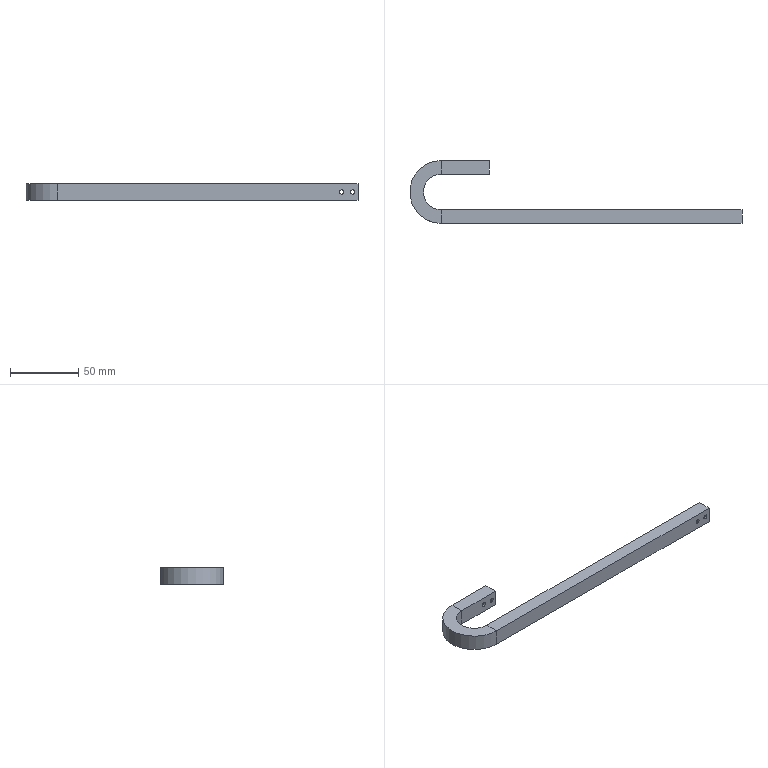Part | NX | features BREP 1 | 1 solid | 46 faces | box 243 x 46 x 12 mm | volume 22023 mm3 | plane 22 | cylinder 20 | cone 4 | commonest cylinder face diameters 3.2 x16 26 x1 29 x1 43 x1 46 x1
STEP:
#1=CARTESIAN_POINT('',(181.,-39.5,-1.6));
#2=VERTEX_POINT('',#1);
#3=CARTESIAN_POINT('',(181.,-40.999,-1.6));
#4=VERTEX_POINT('',#3);
#5=CARTESIAN_POINT('',(181.,-31.,-1.6));
#6=DIRECTION('',(0.,1.,0.));
#7=VECTOR('',#6,1000.);
#8=LINE('',#5,#7);
#9=EDGE_CURVE('',#2,#4,#8,.F.);
#10=ORIENTED_EDGE('',*,*,#9,.T.);
#11=CARTESIAN_POINT('',(181.,-40.999,1.6));
#12=VERTEX_POINT('',#11);
#13=CARTESIAN_POINT('',(181.,-40.999,0.));
#14=DIRECTION('',(0.,1.,0.));
#15=DIRECTION('',(0.,0.,1.));
#16=AXIS2_PLACEMENT_3D('',#13,#14,#15);
#17=CIRCLE('',#16,1.6);
#18=EDGE_CURVE('',#12,#4,#17,.T.);
#19=ORIENTED_EDGE('',*,*,#18,.F.);
#20=CARTESIAN_POINT('',(181.,-39.5,1.6));
#21=VERTEX_POINT('',#20);
#22=CARTESIAN_POINT('',(181.,-31.,1.6));
#23=DIRECTION('',(0.,1.,0.));
#24=VECTOR('',#23,1000.);
#25=LINE('',#22,#24);
#26=EDGE_CURVE('',#21,#12,#25,.F.);
#27=ORIENTED_EDGE('',*,*,#26,.F.);
#28=CARTESIAN_POINT('',(181.,-39.5,0.));
#29=DIRECTION('',(0.,-1.,0.));
#30=DIRECTION('',(1.,0.,0.));
#31=AXIS2_PLACEMENT_3D('',#28,#29,#30);
#32=CIRCLE('',#31,1.6);
#33=EDGE_CURVE('',#2,#21,#32,.T.);
#34=ORIENTED_EDGE('',*,*,#33,.F.);
#35=EDGE_LOOP('',(#10,#19,#27,#34));
#36=FACE_BOUND('',#35,.T.);
#37=CARTESIAN_POINT('',(181.,-31.,0.));
#38=DIRECTION('',(0.,1.,0.));
#39=DIRECTION('',(0.,0.,1.));
#40=AXIS2_PLACEMENT_3D('',#37,#38,#39);
#41=CYLINDRICAL_SURFACE('',#40,1.6);
#42=ADVANCED_FACE('',(#36),#41,.F.);
#43=CARTESIAN_POINT('',(181.,-41.,-1.598));
#44=VERTEX_POINT('',#43);
#45=CARTESIAN_POINT('',(181.,-40.999,-1.6));
#46=DIRECTION('',(0.,0.515,-0.8572));
#47=VECTOR('',#46,1000.);
#48=LINE('',#45,#47);
#49=EDGE_CURVE('',#4,#44,#48,.F.);
#50=ORIENTED_EDGE('',*,*,#49,.T.);
#51=CARTESIAN_POINT('',(181.,-41.,1.598));
#52=VERTEX_POINT('',#51);
#53=CARTESIAN_POINT('',(181.,-41.,0.));
#54=DIRECTION('',(0.,1.,0.));
#55=DIRECTION('',(-1.,0.,0.));
#56=AXIS2_PLACEMENT_3D('',#53,#54,#55);
#57=CIRCLE('',#56,1.598);
#58=EDGE_CURVE('',#52,#44,#57,.T.);
#59=ORIENTED_EDGE('',*,*,#58,.F.);
#60=CARTESIAN_POINT('',(181.,-40.999,1.6));
#61=DIRECTION('',(0.,0.515,0.8572));
#62=VECTOR('',#61,1000.);
#63=LINE('',#60,#62);
#64=EDGE_CURVE('',#12,#52,#63,.F.);
#65=ORIENTED_EDGE('',*,*,#64,.F.);
#66=ORIENTED_EDGE('',*,*,#18,.T.);
#67=EDGE_LOOP('',(#50,#59,#65,#66));
#68=FACE_BOUND('',#67,.T.);
#69=CARTESIAN_POINT('',(181.,-40.999,0.));
#70=DIRECTION('',(0.,1.,0.));
#71=DIRECTION('',(0.,0.,1.));
#72=AXIS2_PLACEMENT_3D('',#69,#70,#71);
#73=CONICAL_SURFACE('',#72,1.6,1.03);
#74=ADVANCED_FACE('',(#68),#73,.F.);
#75=CARTESIAN_POINT('',(181.,-31.,-1.6));
#76=VERTEX_POINT('',#75);
#77=CARTESIAN_POINT('',(181.,-32.5,-1.6));
#78=VERTEX_POINT('',#77);
#79=CARTESIAN_POINT('',(181.,-31.,-1.6));
#80=DIRECTION('',(0.,1.,0.));
#81=VECTOR('',#80,1000.);
#82=LINE('',#79,#81);
#83=EDGE_CURVE('',#76,#78,#82,.F.);
#84=ORIENTED_EDGE('',*,*,#83,.T.);
#85=CARTESIAN_POINT('',(181.,-32.5,1.6));
#86=VERTEX_POINT('',#85);
#87=CARTESIAN_POINT('',(181.,-32.5,0.));
#88=DIRECTION('',(0.,1.,0.));
#89=DIRECTION('',(-1.,0.,0.));
#90=AXIS2_PLACEMENT_3D('',#87,#88,#89);
#91=CIRCLE('',#90,1.6);
#92=EDGE_CURVE('',#86,#78,#91,.T.);
#93=ORIENTED_EDGE('',*,*,#92,.F.);
#94=CARTESIAN_POINT('',(181.,-31.,1.6));
#95=VERTEX_POINT('',#94);
#96=CARTESIAN_POINT('',(181.,-31.,1.6));
#97=DIRECTION('',(0.,1.,0.));
#98=VECTOR('',#97,1000.);
#99=LINE('',#96,#98);
#100=EDGE_CURVE('',#95,#86,#99,.F.);
#101=ORIENTED_EDGE('',*,*,#100,.F.);
#102=CARTESIAN_POINT('',(181.,-31.,0.));
#103=DIRECTION('',(0.,1.,0.));
#104=DIRECTION('',(0.,0.,1.));
#105=AXIS2_PLACEMENT_3D('',#102,#103,#104);
#106=CIRCLE('',#105,1.6);
#107=EDGE_CURVE('',#95,#76,#106,.T.);
#108=ORIENTED_EDGE('',*,*,#107,.T.);
#109=EDGE_LOOP('',(#84,#93,#101,#108));
#110=FACE_BOUND('',#109,.T.);
#111=CARTESIAN_POINT('',(181.,-31.,0.));
#112=DIRECTION('',(0.,1.,0.));
#113=DIRECTION('',(0.,0.,1.));
#114=AXIS2_PLACEMENT_3D('',#111,#112,#113);
#115=CYLINDRICAL_SURFACE('',#114,1.6);
#116=ADVANCED_FACE('',(#110),#115,.F.);
#117=CARTESIAN_POINT('',(173.,-39.5,-1.6));
#118=VERTEX_POINT('',#117);
#119=CARTESIAN_POINT('',(173.,-40.999,-1.6));
#120=VERTEX_POINT('',#119);
#121=CARTESIAN_POINT('',(173.,-31.,-1.6));
#122=DIRECTION('',(0.,1.,0.));
#123=VECTOR('',#122,1000.);
#124=LINE('',#121,#123);
#125=EDGE_CURVE('',#118,#120,#124,.F.);
#126=ORIENTED_EDGE('',*,*,#125,.T.);
#127=CARTESIAN_POINT('',(173.,-40.999,1.6));
#128=VERTEX_POINT('',#127);
#129=CARTESIAN_POINT('',(173.,-40.999,0.));
#130=DIRECTION('',(0.,1.,0.));
#131=DIRECTION('',(0.,0.,1.));
#132=AXIS2_PLACEMENT_3D('',#129,#130,#131);
#133=CIRCLE('',#132,1.6);
#134=EDGE_CURVE('',#128,#120,#133,.T.);
#135=ORIENTED_EDGE('',*,*,#134,.F.);
#136=CARTESIAN_POINT('',(173.,-39.5,1.6));
#137=VERTEX_POINT('',#136);
#138=CARTESIAN_POINT('',(173.,-31.,1.6));
#139=DIRECTION('',(0.,1.,0.));
#140=VECTOR('',#139,1000.);
#141=LINE('',#138,#140);
#142=EDGE_CURVE('',#137,#128,#141,.F.);
#143=ORIENTED_EDGE('',*,*,#142,.F.);
#144=CARTESIAN_POINT('',(173.,-39.5,0.));
#145=DIRECTION('',(0.,-1.,0.));
#146=DIRECTION('',(1.,0.,0.));
#147=AXIS2_PLACEMENT_3D('',#144,#145,#146);
#148=CIRCLE('',#147,1.6);
#149=EDGE_CURVE('',#118,#137,#148,.T.);
#150=ORIENTED_EDGE('',*,*,#149,.F.);
#151=EDGE_LOOP('',(#126,#135,#143,#150));
#152=FACE_BOUND('',#151,.T.);
#153=CARTESIAN_POINT('',(173.,-31.,0.));
#154=DIRECTION('',(0.,1.,0.));
#155=DIRECTION('',(0.,0.,1.));
#156=AXIS2_PLACEMENT_3D('',#153,#154,#155);
#157=CYLINDRICAL_SURFACE('',#156,1.6);
#158=ADVANCED_FACE('',(#152),#157,.F.);
#159=CARTESIAN_POINT('',(173.,-41.,-1.598));
#160=VERTEX_POINT('',#159);
#161=CARTESIAN_POINT('',(173.,-40.999,-1.6));
#162=DIRECTION('',(0.,0.515,-0.8572));
#163=VECTOR('',#162,1000.);
#164=LINE('',#161,#163);
#165=EDGE_CURVE('',#120,#160,#164,.F.);
#166=ORIENTED_EDGE('',*,*,#165,.T.);
#167=CARTESIAN_POINT('',(173.,-41.,1.598));
#168=VERTEX_POINT('',#167);
#169=CARTESIAN_POINT('',(173.,-41.,0.));
#170=DIRECTION('',(0.,1.,0.));
#171=DIRECTION('',(-1.,0.,0.));
#172=AXIS2_PLACEMENT_3D('',#169,#170,#171);
#173=CIRCLE('',#172,1.598);
#174=EDGE_CURVE('',#168,#160,#173,.T.);
#175=ORIENTED_EDGE('',*,*,#174,.F.);
#176=CARTESIAN_POINT('',(173.,-40.999,1.6));
#177=DIRECTION('',(0.,0.515,0.8572));
#178=VECTOR('',#177,1000.);
#179=LINE('',#176,#178);
#180=EDGE_CURVE('',#128,#168,#179,.F.);
#181=ORIENTED_EDGE('',*,*,#180,.F.);
#182=ORIENTED_EDGE('',*,*,#134,.T.);
#183=EDGE_LOOP('',(#166,#175,#181,#182));
#184=FACE_BOUND('',#183,.T.);
#185=CARTESIAN_POINT('',(173.,-40.999,0.));
#186=DIRECTION('',(0.,1.,0.));
#187=DIRECTION('',(0.,0.,1.));
#188=AXIS2_PLACEMENT_3D('',#185,#186,#187);
#189=CONICAL_SURFACE('',#188,1.6,1.03);
#190=ADVANCED_FACE('',(#184),#189,.F.);
#191=CARTESIAN_POINT('',(173.,-31.,-1.6));
#192=VERTEX_POINT('',#191);
#193=CARTESIAN_POINT('',(173.,-32.5,-1.6));
#194=VERTEX_POINT('',#193);
#195=CARTESIAN_POINT('',(173.,-31.,-1.6));
#196=DIRECTION('',(0.,1.,0.));
#197=VECTOR('',#196,1000.);
#198=LINE('',#195,#197);
#199=EDGE_CURVE('',#192,#194,#198,.F.);
#200=ORIENTED_EDGE('',*,*,#199,.T.);
#201=CARTESIAN_POINT('',(173.,-32.5,1.6));
#202=VERTEX_POINT('',#201);
#203=CARTESIAN_POINT('',(173.,-32.5,0.));
#204=DIRECTION('',(0.,1.,0.));
#205=DIRECTION('',(-1.,0.,0.));
#206=AXIS2_PLACEMENT_3D('',#203,#204,#205);
#207=CIRCLE('',#206,1.6);
#208=EDGE_CURVE('',#202,#194,#207,.T.);
#209=ORIENTED_EDGE('',*,*,#208,.F.);
#210=CARTESIAN_POINT('',(173.,-31.,1.6));
#211=VERTEX_POINT('',#210);
#212=CARTESIAN_POINT('',(173.,-31.,1.6));
#213=DIRECTION('',(0.,1.,0.));
#214=VECTOR('',#213,1000.);
#215=LINE('',#212,#214);
#216=EDGE_CURVE('',#211,#202,#215,.F.);
#217=ORIENTED_EDGE('',*,*,#216,.F.);
#218=CARTESIAN_POINT('',(173.,-31.,0.));
#219=DIRECTION('',(0.,1.,0.));
#220=DIRECTION('',(0.,0.,1.));
#221=AXIS2_PLACEMENT_3D('',#218,#219,#220);
#222=CIRCLE('',#221,1.6);
#223=EDGE_CURVE('',#211,#192,#222,.T.);
#224=ORIENTED_EDGE('',*,*,#223,.T.);
#225=EDGE_LOOP('',(#200,#209,#217,#224));
#226=FACE_BOUND('',#225,.T.);
#227=CARTESIAN_POINT('',(173.,-31.,0.));
#228=DIRECTION('',(0.,1.,0.));
#229=DIRECTION('',(0.,0.,1.));
#230=AXIS2_PLACEMENT_3D('',#227,#228,#229);
#231=CYLINDRICAL_SURFACE('',#230,1.6);
#232=ADVANCED_FACE('',(#226),#231,.F.);
#233=CARTESIAN_POINT('',(-4.,-3.5,-1.6));
#234=VERTEX_POINT('',#233);
#235=CARTESIAN_POINT('',(-4.,-5.,-1.6));
#236=VERTEX_POINT('',#235);
#237=CARTESIAN_POINT('',(-4.,5.,-1.6));
#238=DIRECTION('',(0.,1.,0.));
#239=VECTOR('',#238,1000.);
#240=LINE('',#237,#239);
#241=EDGE_CURVE('',#234,#236,#240,.F.);
#242=ORIENTED_EDGE('',*,*,#241,.T.);
#243=CARTESIAN_POINT('',(-4.,-5.,1.6));
#244=VERTEX_POINT('',#243);
#245=CARTESIAN_POINT('',(-4.,-5.,0.));
#246=DIRECTION('',(0.,-1.,0.));
#247=DIRECTION('',(-1.,0.,0.));
#248=AXIS2_PLACEMENT_3D('',#245,#246,#247);
#249=CIRCLE('',#248,1.6);
#250=EDGE_CURVE('',#236,#244,#249,.T.);
#251=ORIENTED_EDGE('',*,*,#250,.T.);
#252=CARTESIAN_POINT('',(-4.,-3.5,1.6));
#253=VERTEX_POINT('',#252);
#254=CARTESIAN_POINT('',(-4.,5.,1.6));
#255=DIRECTION('',(0.,1.,0.));
#256=VECTOR('',#255,1000.);
#257=LINE('',#254,#256);
#258=EDGE_CURVE('',#253,#244,#257,.F.);
#259=ORIENTED_EDGE('',*,*,#258,.F.);
#260=CARTESIAN_POINT('',(-4.,-3.5,0.));
#261=DIRECTION('',(0.,-1.,0.));
#262=DIRECTION('',(1.,0.,0.));
#263=AXIS2_PLACEMENT_3D('',#260,#261,#262);
#264=CIRCLE('',#263,1.6);
#265=EDGE_CURVE('',#234,#253,#264,.T.);
#266=ORIENTED_EDGE('',*,*,#265,.F.);
#267=EDGE_LOOP('',(#242,#251,#259,#266));
#268=FACE_BOUND('',#267,.T.);
#269=CARTESIAN_POINT('',(-4.,5.,0.));
#270=DIRECTION('',(0.,1.,0.));
#271=DIRECTION('',(0.,0.,1.));
#272=AXIS2_PLACEMENT_3D('',#269,#270,#271);
#273=CYLINDRICAL_SURFACE('',#272,1.6);
#274=ADVANCED_FACE('',(#268),#273,.F.);
#275=CARTESIAN_POINT('',(-4.,5.,-1.6));
#276=VERTEX_POINT('',#275);
#277=CARTESIAN_POINT('',(-4.,3.5,-1.6));
#278=VERTEX_POINT('',#277);
#279=CARTESIAN_POINT('',(-4.,5.,-1.6));
#280=DIRECTION('',(0.,1.,0.));
#281=VECTOR('',#280,1000.);
#282=LINE('',#279,#281);
#283=EDGE_CURVE('',#276,#278,#282,.F.);
#284=ORIENTED_EDGE('',*,*,#283,.T.);
#285=CARTESIAN_POINT('',(-4.,3.5,1.6));
#286=VERTEX_POINT('',#285);
#287=CARTESIAN_POINT('',(-4.,3.5,0.));
#288=DIRECTION('',(0.,1.,0.));
#289=DIRECTION('',(-1.,0.,0.));
#290=AXIS2_PLACEMENT_3D('',#287,#288,#289);
#291=CIRCLE('',#290,1.6);
#292=EDGE_CURVE('',#286,#278,#291,.T.);
#293=ORIENTED_EDGE('',*,*,#292,.F.);
#294=CARTESIAN_POINT('',(-4.,5.,1.6));
#295=VERTEX_POINT('',#294);
#296=CARTESIAN_POINT('',(-4.,5.,1.6));
#297=DIRECTION('',(0.,1.,0.));
#298=VECTOR('',#297,1000.);
#299=LINE('',#296,#298);
#300=EDGE_CURVE('',#295,#286,#299,.F.);
#301=ORIENTED_EDGE('',*,*,#300,.F.);
#302=CARTESIAN_POINT('',(-4.,5.,0.));
#303=DIRECTION('',(0.,1.,0.));
#304=DIRECTION('',(0.,0.,1.));
#305=AXIS2_PLACEMENT_3D('',#302,#303,#304);
#306=CIRCLE('',#305,1.6);
#307=EDGE_CURVE('',#295,#276,#306,.T.);
#308=ORIENTED_EDGE('',*,*,#307,.T.);
#309=EDGE_LOOP('',(#284,#293,#301,#308));
#310=FACE_BOUND('',#309,.T.);
#311=CARTESIAN_POINT('',(-4.,5.,0.));
#312=DIRECTION('',(0.,1.,0.));
#313=DIRECTION('',(0.,0.,1.));
#314=AXIS2_PLACEMENT_3D('',#311,#312,#313);
#315=CYLINDRICAL_SURFACE('',#314,1.6);
#316=ADVANCED_FACE('',(#310),#315,.F.);
#317=CARTESIAN_POINT('',(-12.,5.,-1.6));
#318=VERTEX_POINT('',#317);
#319=CARTESIAN_POINT('',(-12.,3.5,-1.6));
#320=VERTEX_POINT('',#319);
#321=CARTESIAN_POINT('',(-12.,5.,-1.6));
#322=DIRECTION('',(0.,1.,0.));
#323=VECTOR('',#322,1000.);
#324=LINE('',#321,#323);
#325=EDGE_CURVE('',#318,#320,#324,.F.);
#326=ORIENTED_EDGE('',*,*,#325,.T.);
#327=CARTESIAN_POINT('',(-12.,3.5,1.6));
#328=VERTEX_POINT('',#327);
#329=CARTESIAN_POINT('',(-12.,3.5,0.));
#330=DIRECTION('',(0.,1.,0.));
#331=DIRECTION('',(-1.,0.,0.));
#332=AXIS2_PLACEMENT_3D('',#329,#330,#331);
#333=CIRCLE('',#332,1.6);
#334=EDGE_CURVE('',#328,#320,#333,.T.);
#335=ORIENTED_EDGE('',*,*,#334,.F.);
#336=CARTESIAN_POINT('',(-12.,5.,1.6));
#337=VERTEX_POINT('',#336);
#338=CARTESIAN_POINT('',(-12.,5.,1.6));
#339=DIRECTION('',(0.,1.,0.));
#340=VECTOR('',#339,1000.);
#341=LINE('',#338,#340);
#342=EDGE_CURVE('',#337,#328,#341,.F.);
#343=ORIENTED_EDGE('',*,*,#342,.F.);
#344=CARTESIAN_POINT('',(-12.,5.,0.));
#345=DIRECTION('',(0.,1.,0.));
#346=DIRECTION('',(0.,0.,1.));
#347=AXIS2_PLACEMENT_3D('',#344,#345,#346);
#348=CIRCLE('',#347,1.6);
#349=EDGE_CURVE('',#337,#318,#348,.T.);
#350=ORIENTED_EDGE('',*,*,#349,.T.);
#351=EDGE_LOOP('',(#326,#335,#343,#350));
#352=FACE_BOUND('',#351,.T.);
#353=CARTESIAN_POINT('',(-12.,5.,0.));
#354=DIRECTION('',(0.,1.,0.));
#355=DIRECTION('',(0.,0.,1.));
#356=AXIS2_PLACEMENT_3D('',#353,#354,#355);
#357=CYLINDRICAL_SURFACE('',#356,1.6);
#358=ADVANCED_FACE('',(#352),#357,.F.);
#359=CARTESIAN_POINT('',(-12.,-3.5,-1.6));
#360=VERTEX_POINT('',#359);
#361=CARTESIAN_POINT('',(-12.,-5.,-1.6));
#362=VERTEX_POINT('',#361);
#363=CARTESIAN_POINT('',(-12.,5.,-1.6));
#364=DIRECTION('',(0.,1.,0.));
#365=VECTOR('',#364,1000.);
#366=LINE('',#363,#365);
#367=EDGE_CURVE('',#360,#362,#366,.F.);
#368=ORIENTED_EDGE('',*,*,#367,.T.);
#369=CARTESIAN_POINT('',(-12.,-5.,1.6));
#370=VERTEX_POINT('',#369);
#371=CARTESIAN_POINT('',(-12.,-5.,0.));
#372=DIRECTION('',(0.,-1.,0.));
#373=DIRECTION('',(-1.,0.,0.));
#374=AXIS2_PLACEMENT_3D('',#371,#372,#373);
#375=CIRCLE('',#374,1.6);
#376=EDGE_CURVE('',#362,#370,#375,.T.);
#377=ORIENTED_EDGE('',*,*,#376,.T.);
#378=CARTESIAN_POINT('',(-12.,-3.5,1.6));
#379=VERTEX_POINT('',#378);
#380=CARTESIAN_POINT('',(-12.,5.,1.6));
#381=DIRECTION('',(0.,1.,0.));
#382=VECTOR('',#381,1000.);
#383=LINE('',#380,#382);
#384=EDGE_CURVE('',#379,#370,#383,.F.);
#385=ORIENTED_EDGE('',*,*,#384,.F.);
#386=CARTESIAN_POINT('',(-12.,-3.5,0.));
#387=DIRECTION('',(0.,-1.,0.));
#388=DIRECTION('',(1.,0.,0.));
#389=AXIS2_PLACEMENT_3D('',#386,#387,#388);
#390=CIRCLE('',#389,1.6);
#391=EDGE_CURVE('',#360,#379,#390,.T.);
#392=ORIENTED_EDGE('',*,*,#391,.F.);
#393=EDGE_LOOP('',(#368,#377,#385,#392));
#394=FACE_BOUND('',#393,.T.);
#395=CARTESIAN_POINT('',(-12.,5.,0.));
#396=DIRECTION('',(0.,1.,0.));
#397=DIRECTION('',(0.,0.,1.));
#398=AXIS2_PLACEMENT_3D('',#395,#396,#397);
#399=CYLINDRICAL_SURFACE('',#398,1.6);
#400=ADVANCED_FACE('',(#394),#399,.F.);
#401=CARTESIAN_POINT('',(0.,5.,-6.));
#402=VERTEX_POINT('',#401);
#403=CARTESIAN_POINT('',(-35.,5.,-6.));
#404=VERTEX_POINT('',#403);
#405=CARTESIAN_POINT('',(0.,5.,-6.));
#406=DIRECTION('',(-1.,0.,0.));
#407=VECTOR('',#406,1000.);
#408=LINE('',#405,#407);
#409=EDGE_CURVE('',#402,#404,#408,.T.);
#410=ORIENTED_EDGE('',*,*,#409,.F.);
#411=CARTESIAN_POINT('',(0.,-5.,-6.));
#412=VERTEX_POINT('',#411);
#413=CARTESIAN_POINT('',(0.,-5.,-6.));
#414=DIRECTION('',(0.,1.,0.));
#415=VECTOR('',#414,1000.);
#416=LINE('',#413,#415);
#417=EDGE_CURVE('',#412,#402,#416,.T.);
#418=ORIENTED_EDGE('',*,*,#417,.F.);
#419=CARTESIAN_POINT('',(-35.,-5.,-6.));
#420=VERTEX_POINT('',#419);
#421=CARTESIAN_POINT('',(0.,-5.,-6.));
#422=DIRECTION('',(-1.,0.,0.));
#423=VECTOR('',#422,1000.);
#424=LINE('',#421,#423);
#425=EDGE_CURVE('',#412,#420,#424,.T.);
#426=ORIENTED_EDGE('',*,*,#425,.T.);
#427=CARTESIAN_POINT('',(-35.,-5.,-6.));
#428=DIRECTION('',(0.,1.,0.));
#429=VECTOR('',#428,1000.);
#430=LINE('',#427,#429);
#431=EDGE_CURVE('',#420,#404,#430,.T.);
#432=ORIENTED_EDGE('',*,*,#431,.T.);
#433=EDGE_LOOP('',(#410,#418,#426,#432));
#434=FACE_BOUND('',#433,.T.);
#435=CARTESIAN_POINT('',(0.,-5.,-6.));
#436=DIRECTION('',(0.,0.,1.));
#437=DIRECTION('',(1.,0.,0.));
#438=AXIS2_PLACEMENT_3D('',#435,#436,#437);
#439=PLANE('',#438);
#440=ADVANCED_FACE('',(#434),#439,.F.);
#441=CARTESIAN_POINT('',(0.,5.,6.));
#442=VERTEX_POINT('',#441);
#443=CARTESIAN_POINT('',(-35.,5.,6.));
#444=VERTEX_POINT('',#443);
#445=CARTESIAN_POINT('',(0.,5.,6.));
#446=DIRECTION('',(-1.,0.,0.));
#447=VECTOR('',#446,1000.);
#448=LINE('',#445,#447);
#449=EDGE_CURVE('',#442,#444,#448,.T.);
#450=ORIENTED_EDGE('',*,*,#449,.F.);
#451=CARTESIAN_POINT('',(0.,5.,6.));
#452=DIRECTION('',(0.,0.,1.));
#453=VECTOR('',#452,1000.);
#454=LINE('',#451,#453);
#455=EDGE_CURVE('',#402,#442,#454,.T.);
#456=ORIENTED_EDGE('',*,*,#455,.F.);
#457=ORIENTED_EDGE('',*,*,#409,.T.);
#458=CARTESIAN_POINT('',(-35.,5.,6.));
#459=DIRECTION('',(0.,0.,1.));
#460=VECTOR('',#459,1000.);
#461=LINE('',#458,#460);
#462=EDGE_CURVE('',#404,#444,#461,.T.);
#463=ORIENTED_EDGE('',*,*,#462,.T.);
#464=EDGE_LOOP('',(#450,#456,#457,#463));
#465=FACE_BOUND('',#464,.T.);
#466=ORIENTED_EDGE('',*,*,#349,.F.);
#467=CARTESIAN_POINT('',(-12.,5.,0.));
#468=DIRECTION('',(0.,1.,0.));
#469=DIRECTION('',(0.,0.,1.));
#470=AXIS2_PLACEMENT_3D('',#467,#468,#469);
#471=CIRCLE('',#470,1.6);
#472=EDGE_CURVE('',#318,#337,#471,.T.);
#473=ORIENTED_EDGE('',*,*,#472,.F.);
#474=EDGE_LOOP('',(#466,#473));
#475=FACE_BOUND('',#474,.T.);
#476=ORIENTED_EDGE('',*,*,#307,.F.);
#477=CARTESIAN_POINT('',(-4.,5.,0.));
#478=DIRECTION('',(0.,1.,0.));
#479=DIRECTION('',(0.,0.,1.));
#480=AXIS2_PLACEMENT_3D('',#477,#478,#479);
#481=CIRCLE('',#480,1.6);
#482=EDGE_CURVE('',#276,#295,#481,.T.);
#483=ORIENTED_EDGE('',*,*,#482,.F.);
#484=EDGE_LOOP('',(#476,#483));
#485=FACE_BOUND('',#484,.T.);
#486=CARTESIAN_POINT('',(0.,5.,6.));
#487=DIRECTION('',(0.,-1.,0.));
#488=DIRECTION('',(1.,0.,0.));
#489=AXIS2_PLACEMENT_3D('',#486,#487,#488);
#490=PLANE('',#489);
#491=ADVANCED_FACE('',(#465,#475,#485),#490,.F.);
#492=CARTESIAN_POINT('',(0.,-5.,6.));
#493=VERTEX_POINT('',#492);
#494=CARTESIAN_POINT('',(-35.,-5.,6.));
#495=VERTEX_POINT('',#494);
#496=CARTESIAN_POINT('',(0.,-5.,6.));
#497=DIRECTION('',(-1.,0.,0.));
#498=VECTOR('',#497,1000.);
#499=LINE('',#496,#498);
#500=EDGE_CURVE('',#493,#495,#499,.T.);
#501=ORIENTED_EDGE('',*,*,#500,.F.);
#502=CARTESIAN_POINT('',(0.,-5.,6.));
#503=DIRECTION('',(0.,-1.,0.));
#504=VECTOR('',#503,1000.);
#505=LINE('',#502,#504);
#506=EDGE_CURVE('',#442,#493,#505,.T.);
#507=ORIENTED_EDGE('',*,*,#506,.F.);
#508=ORIENTED_EDGE('',*,*,#449,.T.);
#509=CARTESIAN_POINT('',(-35.,-5.,6.));
#510=DIRECTION('',(0.,-1.,0.));
#511=VECTOR('',#510,1000.);
#512=LINE('',#509,#511);
#513=EDGE_CURVE('',#444,#495,#512,.T.);
#514=ORIENTED_EDGE('',*,*,#513,.T.);
#515=EDGE_LOOP('',(#501,#507,#508,#514));
#516=FACE_BOUND('',#515,.T.);
#517=CARTESIAN_POINT('',(0.,-5.,6.));
#518=DIRECTION('',(0.,0.,-1.));
#519=DIRECTION('',(-1.,0.,0.));
#520=AXIS2_PLACEMENT_3D('',#517,#518,#519);
#521=PLANE('',#520);
#522=ADVANCED_FACE('',(#516),#521,.F.);
#523=CARTESIAN_POINT('',(-35.,-5.,6.));
#524=DIRECTION('',(0.,0.,-1.));
#525=VECTOR('',#524,1000.);
#526=LINE('',#523,#525);
#527=EDGE_CURVE('',#495,#420,#526,.T.);
#528=ORIENTED_EDGE('',*,*,#527,.T.);
#529=ORIENTED_EDGE('',*,*,#425,.F.);
#530=CARTESIAN_POINT('',(0.,-5.,6.));
#531=DIRECTION('',(0.,0.,-1.));
#532=VECTOR('',#531,1000.);
#533=LINE('',#530,#532);
#534=EDGE_CURVE('',#493,#412,#533,.T.);
#535=ORIENTED_EDGE('',*,*,#534,.F.);
#536=ORIENTED_EDGE('',*,*,#500,.T.);
#537=EDGE_LOOP('',(#528,#529,#535,#536));
#538=FACE_BOUND('',#537,.T.);
#539=CARTESIAN_POINT('',(-12.,-5.,0.));
#540=DIRECTION('',(0.,-1.,0.));
#541=DIRECTION('',(-1.,0.,0.));
#542=AXIS2_PLACEMENT_3D('',#539,#540,#541);
#543=CIRCLE('',#542,1.6);
#544=EDGE_CURVE('',#370,#362,#543,.T.);
#545=ORIENTED_EDGE('',*,*,#544,.F.);
#546=ORIENTED_EDGE('',*,*,#376,.F.);
#547=EDGE_LOOP('',(#545,#546));
#548=FACE_BOUND('',#547,.T.);
#549=CARTESIAN_POINT('',(-4.,-5.,0.));
#550=DIRECTION('',(0.,-1.,0.));
#551=DIRECTION('',(-1.,0.,0.));
#552=AXIS2_PLACEMENT_3D('',#549,#550,#551);
#553=CIRCLE('',#552,1.6);
#554=EDGE_CURVE('',#244,#236,#553,.T.);
#555=ORIENTED_EDGE('',*,*,#554,.F.);
#556=ORIENTED_EDGE('',*,*,#250,.F.);
#557=EDGE_LOOP('',(#555,#556));
#558=FACE_BOUND('',#557,.T.);
#559=CARTESIAN_POINT('',(0.,-5.,6.));
#560=DIRECTION('',(0.,1.,0.));
#561=DIRECTION('',(-1.,0.,0.));
#562=AXIS2_PLACEMENT_3D('',#559,#560,#561);
#563=PLANE('',#562);
#564=ADVANCED_FACE('',(#538,#548,#558),#563,.F.);
#565=CARTESIAN_POINT('',(-35.,-41.,-6.));
#566=VERTEX_POINT('',#565);
#567=CARTESIAN_POINT('',(-35.,-18.,-6.));
#568=DIRECTION('',(0.,0.,1.));
#569=DIRECTION('',(0.,1.,0.));
#570=AXIS2_PLACEMENT_3D('',#567,#568,#569);
#571=CIRCLE('',#570,23.);
#572=EDGE_CURVE('',#404,#566,#571,.T.);
#573=ORIENTED_EDGE('',*,*,#572,.F.);
#574=ORIENTED_EDGE('',*,*,#431,.F.);
#575=CARTESIAN_POINT('',(-35.,-31.,-6.));
#576=VERTEX_POINT('',#575);
#577=CARTESIAN_POINT('',(-35.,-18.,-6.));
#578=DIRECTION('',(0.,0.,1.));
#579=DIRECTION('',(0.,1.,0.));
#580=AXIS2_PLACEMENT_3D('',#577,#578,#579);
#581=CIRCLE('',#580,13.);
#582=EDGE_CURVE('',#420,#576,#581,.T.);
#583=ORIENTED_EDGE('',*,*,#582,.T.);
#584=CARTESIAN_POINT('',(-35.,-31.,-6.));
#585=DIRECTION('',(0.,-1.,0.));
#586=VECTOR('',#585,1000.);
#587=LINE('',#584,#586);
#588=EDGE_CURVE('',#576,#566,#587,.T.);
#589=ORIENTED_EDGE('',*,*,#588,.T.);
#590=EDGE_LOOP('',(#573,#574,#583,#589));
#591=FACE_BOUND('',#590,.T.);
#592=CARTESIAN_POINT('',(-35.,-5.,-6.));
#593=DIRECTION('',(0.,0.,1.));
#594=DIRECTION('',(1.,0.,0.));
#595=AXIS2_PLACEMENT_3D('',#592,#593,#594);
#596=PLANE('',#595);
#597=ADVANCED_FACE('',(#591),#596,.F.);
#598=CARTESIAN_POINT('',(-35.,-41.,6.));
#599=VERTEX_POINT('',#598);
#600=CARTESIAN_POINT('',(-35.,-18.,6.));
#601=DIRECTION('',(0.,0.,1.));
#602=DIRECTION('',(0.,1.,0.));
#603=AXIS2_PLACEMENT_3D('',#600,#601,#602);
#604=CIRCLE('',#603,23.);
#605=EDGE_CURVE('',#444,#599,#604,.T.);
#606=ORIENTED_EDGE('',*,*,#605,.F.);
#607=ORIENTED_EDGE('',*,*,#462,.F.);
#608=ORIENTED_EDGE('',*,*,#572,.T.);
#609=CARTESIAN_POINT('',(-35.,-41.,6.));
#610=DIRECTION('',(0.,0.,1.));
#611=VECTOR('',#610,1000.);
#612=LINE('',#609,#611);
#613=EDGE_CURVE('',#566,#599,#612,.T.);
#614=ORIENTED_EDGE('',*,*,#613,.T.);
#615=EDGE_LOOP('',(#606,#607,#608,#614));
#616=FACE_BOUND('',#615,.T.);
#617=CARTESIAN_POINT('',(-35.,-18.,0.));
#618=DIRECTION('',(0.,0.,1.));
#619=DIRECTION('',(1.,0.,0.));
#620=AXIS2_PLACEMENT_3D('',#617,#618,#619);
#621=CYLINDRICAL_SURFACE('',#620,23.);
#622=ADVANCED_FACE('',(#616),#621,.T.);
#623=CARTESIAN_POINT('',(-35.,-31.,6.));
#624=VERTEX_POINT('',#623);
#625=CARTESIAN_POINT('',(-35.,-18.,6.));
#626=DIRECTION('',(0.,0.,1.));
#627=DIRECTION('',(0.,1.,0.));
#628=AXIS2_PLACEMENT_3D('',#625,#626,#627);
#629=CIRCLE('',#628,13.);
#630=EDGE_CURVE('',#495,#624,#629,.T.);
#631=ORIENTED_EDGE('',*,*,#630,.F.);
#632=ORIENTED_EDGE('',*,*,#513,.F.);
#633=ORIENTED_EDGE('',*,*,#605,.T.);
#634=CARTESIAN_POINT('',(-35.,-31.,6.));
#635=DIRECTION('',(0.,1.,0.));
#636=VECTOR('',#635,1000.);
#637=LINE('',#634,#636);
#638=EDGE_CURVE('',#599,#624,#637,.T.);
#639=ORIENTED_EDGE('',*,*,#638,.T.);
#640=EDGE_LOOP('',(#631,#632,#633,#639));
#641=FACE_BOUND('',#640,.T.);
#642=CARTESIAN_POINT('',(-35.,-5.,6.));
#643=DIRECTION('',(0.,0.,-1.));
#644=DIRECTION('',(-1.,0.,0.));
#645=AXIS2_PLACEMENT_3D('',#642,#643,#644);
#646=PLANE('',#645);
#647=ADVANCED_FACE('',(#641),#646,.F.);
#648=CARTESIAN_POINT('',(-35.,-31.,6.));
#649=DIRECTION('',(0.,0.,-1.));
#650=VECTOR('',#649,1000.);
#651=LINE('',#648,#650);
#652=EDGE_CURVE('',#624,#576,#651,.T.);
#653=ORIENTED_EDGE('',*,*,#652,.T.);
#654=ORIENTED_EDGE('',*,*,#582,.F.);
#655=ORIENTED_EDGE('',*,*,#527,.F.);
#656=ORIENTED_EDGE('',*,*,#630,.T.);
#657=EDGE_LOOP('',(#653,#654,#655,#656));
#658=FACE_BOUND('',#657,.T.);
#659=CARTESIAN_POINT('',(-35.,-18.,0.));
#660=DIRECTION('',(0.,0.,1.));
#661=DIRECTION('',(1.,0.,0.));
#662=AXIS2_PLACEMENT_3D('',#659,#660,#661);
#663=CYLINDRICAL_SURFACE('',#662,13.);
#664=ADVANCED_FACE('',(#658),#663,.F.);
#665=CARTESIAN_POINT('',(185.,-41.,-6.));
#666=VERTEX_POINT('',#665);
#667=CARTESIAN_POINT('',(-35.,-41.,-6.));
#668=DIRECTION('',(1.,0.,0.));
#669=VECTOR('',#668,1000.);
#670=LINE('',#667,#669);
#671=EDGE_CURVE('',#566,#666,#670,.T.);
#672=ORIENTED_EDGE('',*,*,#671,.F.);
#673=ORIENTED_EDGE('',*,*,#588,.F.);
#674=CARTESIAN_POINT('',(185.,-31.,-6.));
#675=VERTEX_POINT('',#674);
#676=CARTESIAN_POINT('',(-35.,-31.,-6.));
#677=DIRECTION('',(1.,0.,0.));
#678=VECTOR('',#677,1000.);
#679=LINE('',#676,#678);
#680=EDGE_CURVE('',#576,#675,#679,.T.);
#681=ORIENTED_EDGE('',*,*,#680,.T.);
#682=CARTESIAN_POINT('',(185.,-31.,-6.));
#683=DIRECTION('',(0.,-1.,0.));
#684=VECTOR('',#683,1000.);
#685=LINE('',#682,#684);
#686=EDGE_CURVE('',#675,#666,#685,.T.);
#687=ORIENTED_EDGE('',*,*,#686,.T.);
#688=EDGE_LOOP('',(#672,#673,#681,#687));
#689=FACE_BOUND('',#688,.T.);
#690=CARTESIAN_POINT('',(-35.,-31.,-6.));
#691=DIRECTION('',(0.,0.,1.));
#692=DIRECTION('',(1.,0.,0.));
#693=AXIS2_PLACEMENT_3D('',#690,#691,#692);
#694=PLANE('',#693);
#695=ADVANCED_FACE('',(#689),#694,.F.);
#696=CARTESIAN_POINT('',(185.,-41.,6.));
#697=VERTEX_POINT('',#696);
#698=CARTESIAN_POINT('',(-35.,-41.,6.));
#699=DIRECTION('',(1.,0.,0.));
#700=VECTOR('',#699,1000.);
#701=LINE('',#698,#700);
#702=EDGE_CURVE('',#599,#697,#701,.T.);
#703=ORIENTED_EDGE('',*,*,#702,.F.);
#704=ORIENTED_EDGE('',*,*,#613,.F.);
#705=ORIENTED_EDGE('',*,*,#671,.T.);
#706=CARTESIAN_POINT('',(185.,-41.,6.));
#707=DIRECTION('',(0.,0.,1.));
#708=VECTOR('',#707,1000.);
#709=LINE('',#706,#708);
#710=EDGE_CURVE('',#666,#697,#709,.T.);
#711=ORIENTED_EDGE('',*,*,#710,.T.);
#712=EDGE_LOOP('',(#703,#704,#705,#711));
#713=FACE_BOUND('',#712,.T.);
#714=ORIENTED_EDGE('',*,*,#174,.T.);
#715=CARTESIAN_POINT('',(173.,-41.,0.));
#716=DIRECTION('',(0.,1.,0.));
#717=DIRECTION('',(-1.,0.,0.));
#718=AXIS2_PLACEMENT_3D('',#715,#716,#717);
#719=CIRCLE('',#718,1.598);
#720=EDGE_CURVE('',#160,#168,#719,.T.);
#721=ORIENTED_EDGE('',*,*,#720,.T.);
#722=EDGE_LOOP('',(#714,#721));
#723=FACE_BOUND('',#722,.T.);
#724=ORIENTED_EDGE('',*,*,#58,.T.);
#725=CARTESIAN_POINT('',(181.,-41.,0.));
#726=DIRECTION('',(0.,1.,0.));
#727=DIRECTION('',(-1.,0.,0.));
#728=AXIS2_PLACEMENT_3D('',#725,#726,#727);
#729=CIRCLE('',#728,1.598);
#730=EDGE_CURVE('',#44,#52,#729,.T.);
#731=ORIENTED_EDGE('',*,*,#730,.T.);
#732=EDGE_LOOP('',(#724,#731));
#733=FACE_BOUND('',#732,.T.);
#734=CARTESIAN_POINT('',(-35.,-41.,6.));
#735=DIRECTION('',(0.,1.,0.));
#736=DIRECTION('',(-1.,0.,0.));
#737=AXIS2_PLACEMENT_3D('',#734,#735,#736);
#738=PLANE('',#737);
#739=ADVANCED_FACE('',(#713,#723,#733),#738,.F.);
#740=CARTESIAN_POINT('',(185.,-31.,6.));
#741=VERTEX_POINT('',#740);
#742=CARTESIAN_POINT('',(-35.,-31.,6.));
#743=DIRECTION('',(1.,0.,0.));
#744=VECTOR('',#743,1000.);
#745=LINE('',#742,#744);
#746=EDGE_CURVE('',#624,#741,#745,.T.);
#747=ORIENTED_EDGE('',*,*,#746,.F.);
#748=ORIENTED_EDGE('',*,*,#638,.F.);
#749=ORIENTED_EDGE('',*,*,#702,.T.);
#750=CARTESIAN_POINT('',(185.,-31.,6.));
#751=DIRECTION('',(0.,1.,0.));
#752=VECTOR('',#751,1000.);
#753=LINE('',#750,#752);
#754=EDGE_CURVE('',#697,#741,#753,.T.);
#755=ORIENTED_EDGE('',*,*,#754,.T.);
#756=EDGE_LOOP('',(#747,#748,#749,#755));
#757=FACE_BOUND('',#756,.T.);
#758=CARTESIAN_POINT('',(-35.,-31.,6.));
#759=DIRECTION('',(0.,0.,-1.));
#760=DIRECTION('',(-1.,0.,0.));
#761=AXIS2_PLACEMENT_3D('',#758,#759,#760);
#762=PLANE('',#761);
#763=ADVANCED_FACE('',(#757),#762,.F.);
#764=CARTESIAN_POINT('',(185.,-31.,6.));
#765=DIRECTION('',(0.,0.,-1.));
#766=VECTOR('',#765,1000.);
#767=LINE('',#764,#766);
#768=EDGE_CURVE('',#741,#675,#767,.T.);
#769=ORIENTED_EDGE('',*,*,#768,.T.);
#770=ORIENTED_EDGE('',*,*,#680,.F.);
#771=ORIENTED_EDGE('',*,*,#652,.F.);
#772=ORIENTED_EDGE('',*,*,#746,.T.);
#773=EDGE_LOOP('',(#769,#770,#771,#772));
#774=FACE_BOUND('',#773,.T.);
#775=ORIENTED_EDGE('',*,*,#223,.F.);
#776=CARTESIAN_POINT('',(173.,-31.,0.));
#777=DIRECTION('',(0.,1.,0.));
#778=DIRECTION('',(0.,0.,1.));
#779=AXIS2_PLACEMENT_3D('',#776,#777,#778);
#780=CIRCLE('',#779,1.6);
#781=EDGE_CURVE('',#192,#211,#780,.T.);
#782=ORIENTED_EDGE('',*,*,#781,.F.);
#783=EDGE_LOOP('',(#775,#782));
#784=FACE_BOUND('',#783,.T.);
#785=ORIENTED_EDGE('',*,*,#107,.F.);
#786=CARTESIAN_POINT('',(181.,-31.,0.));
#787=DIRECTION('',(0.,1.,0.));
#788=DIRECTION('',(0.,0.,1.));
#789=AXIS2_PLACEMENT_3D('',#786,#787,#788);
#790=CIRCLE('',#789,1.6);
#791=EDGE_CURVE('',#76,#95,#790,.T.);
#792=ORIENTED_EDGE('',*,*,#791,.F.);
#793=EDGE_LOOP('',(#785,#792));
#794=FACE_BOUND('',#793,.T.);
#795=CARTESIAN_POINT('',(-35.,-31.,6.));
#796=DIRECTION('',(0.,-1.,0.));
#797=DIRECTION('',(1.,0.,0.));
#798=AXIS2_PLACEMENT_3D('',#795,#796,#797);
#799=PLANE('',#798);
#800=ADVANCED_FACE('',(#774,#784,#794),#799,.F.);
#801=CARTESIAN_POINT('',(0.,3.5,-3.5));
#802=VERTEX_POINT('',#801);
#803=CARTESIAN_POINT('',(0.,-3.5,-3.5));
#804=VERTEX_POINT('',#803);
#805=CARTESIAN_POINT('',(0.,-3.5,-3.5));
#806=DIRECTION('',(0.,-1.,0.));
#807=VECTOR('',#806,1000.);
#808=LINE('',#805,#807);
#809=EDGE_CURVE('',#802,#804,#808,.T.);
#810=ORIENTED_EDGE('',*,*,#809,.T.);
#811=CARTESIAN_POINT('',(0.,-3.5,3.5));
#812=VERTEX_POINT('',#811);
#813=CARTESIAN_POINT('',(0.,-3.5,3.5));
#814=DIRECTION('',(0.,0.,1.));
#815=VECTOR('',#814,1000.);
#816=LINE('',#813,#815);
#817=EDGE_CURVE('',#804,#812,#816,.T.);
#818=ORIENTED_EDGE('',*,*,#817,.T.);
#819=CARTESIAN_POINT('',(0.,3.5,3.5));
#820=VERTEX_POINT('',#819);
#821=CARTESIAN_POINT('',(0.,-3.5,3.5));
#822=DIRECTION('',(0.,1.,0.));
#823=VECTOR('',#822,1000.);
#824=LINE('',#821,#823);
#825=EDGE_CURVE('',#812,#820,#824,.T.);
#826=ORIENTED_EDGE('',*,*,#825,.T.);
#827=CARTESIAN_POINT('',(0.,3.5,3.5));
#828=DIRECTION('',(0.,0.,-1.));
#829=VECTOR('',#828,1000.);
#830=LINE('',#827,#829);
#831=EDGE_CURVE('',#820,#802,#830,.T.);
#832=ORIENTED_EDGE('',*,*,#831,.T.);
#833=EDGE_LOOP('',(#810,#818,#826,#832));
#834=FACE_BOUND('',#833,.T.);
#835=ORIENTED_EDGE('',*,*,#417,.T.);
#836=ORIENTED_EDGE('',*,*,#455,.T.);
#837=ORIENTED_EDGE('',*,*,#506,.T.);
#838=ORIENTED_EDGE('',*,*,#534,.T.);
#839=EDGE_LOOP('',(#835,#836,#837,#838));
#840=FACE_BOUND('',#839,.T.);
#841=CARTESIAN_POINT('',(0.,0.,0.));
#842=DIRECTION('',(-1.,0.,0.));
#843=DIRECTION('',(0.,0.,1.));
#844=AXIS2_PLACEMENT_3D('',#841,#842,#843);
#845=PLANE('',#844);
#846=ADVANCED_FACE('',(#834,#840),#845,.F.);
#847=CARTESIAN_POINT('',(185.,-39.5,-3.5));
#848=VERTEX_POINT('',#847);
#849=CARTESIAN_POINT('',(185.,-32.5,-3.5));
#850=VERTEX_POINT('',#849);
#851=CARTESIAN_POINT('',(185.,-32.5,-3.5));
#852=DIRECTION('',(0.,1.,0.));
#853=VECTOR('',#852,1000.);
#854=LINE('',#851,#853);
#855=EDGE_CURVE('',#848,#850,#854,.T.);
#856=ORIENTED_EDGE('',*,*,#855,.F.);
#857=CARTESIAN_POINT('',(185.,-39.5,3.5));
#858=VERTEX_POINT('',#857);
#859=CARTESIAN_POINT('',(185.,-39.5,3.5));
#860=DIRECTION('',(0.,0.,-1.));
#861=VECTOR('',#860,1000.);
#862=LINE('',#859,#861);
#863=EDGE_CURVE('',#858,#848,#862,.T.);
#864=ORIENTED_EDGE('',*,*,#863,.F.);
#865=CARTESIAN_POINT('',(185.,-32.5,3.5));
#866=VERTEX_POINT('',#865);
#867=CARTESIAN_POINT('',(185.,-32.5,3.5));
#868=DIRECTION('',(0.,-1.,0.));
#869=VECTOR('',#868,1000.);
#870=LINE('',#867,#869);
#871=EDGE_CURVE('',#866,#858,#870,.T.);
#872=ORIENTED_EDGE('',*,*,#871,.F.);
#873=CARTESIAN_POINT('',(185.,-32.5,3.5));
#874=DIRECTION('',(0.,0.,1.));
#875=VECTOR('',#874,1000.);
#876=LINE('',#873,#875);
#877=EDGE_CURVE('',#850,#866,#876,.T.);
#878=ORIENTED_EDGE('',*,*,#877,.F.);
#879=EDGE_LOOP('',(#856,#864,#872,#878));
#880=FACE_BOUND('',#879,.T.);
#881=ORIENTED_EDGE('',*,*,#686,.F.);
#882=ORIENTED_EDGE('',*,*,#768,.F.);
#883=ORIENTED_EDGE('',*,*,#754,.F.);
#884=ORIENTED_EDGE('',*,*,#710,.F.);
#885=EDGE_LOOP('',(#881,#882,#883,#884));
#886=FACE_BOUND('',#885,.T.);
#887=CARTESIAN_POINT('',(185.,-36.,0.));
#888=DIRECTION('',(1.,0.,0.));
#889=DIRECTION('',(0.,0.,1.));
#890=AXIS2_PLACEMENT_3D('',#887,#888,#889);
#891=PLANE('',#890);
#892=ADVANCED_FACE('',(#880,#886),#891,.T.);
#893=CARTESIAN_POINT('',(-35.,-3.5,3.5));
#894=VERTEX_POINT('',#893);
#895=CARTESIAN_POINT('',(0.,-3.5,3.5));
#896=DIRECTION('',(-1.,0.,0.));
#897=VECTOR('',#896,1000.);
#898=LINE('',#895,#897);
#899=EDGE_CURVE('',#812,#894,#898,.T.);
#900=ORIENTED_EDGE('',*,*,#899,.F.);
#901=ORIENTED_EDGE('',*,*,#817,.F.);
#902=CARTESIAN_POINT('',(-35.,-3.5,-3.5));
#903=VERTEX_POINT('',#902);
#904=CARTESIAN_POINT('',(0.,-3.5,-3.5));
#905=DIRECTION('',(-1.,0.,0.));
#906=VECTOR('',#905,1000.);
#907=LINE('',#904,#906);
#908=EDGE_CURVE('',#804,#903,#907,.T.);
#909=ORIENTED_EDGE('',*,*,#908,.T.);
#910=CARTESIAN_POINT('',(-35.,-3.5,3.5));
#911=DIRECTION('',(0.,0.,1.));
#912=VECTOR('',#911,1000.);
#913=LINE('',#910,#912);
#914=EDGE_CURVE('',#903,#894,#913,.T.);
#915=ORIENTED_EDGE('',*,*,#914,.T.);
#916=EDGE_LOOP('',(#900,#901,#909,#915));
#917=FACE_BOUND('',#916,.T.);
#918=CARTESIAN_POINT('',(-12.,-3.5,0.));
#919=DIRECTION('',(0.,-1.,0.));
#920=DIRECTION('',(1.,0.,0.));
#921=AXIS2_PLACEMENT_3D('',#918,#919,#920);
#922=CIRCLE('',#921,1.6);
#923=EDGE_CURVE('',#379,#360,#922,.T.);
#924=ORIENTED_EDGE('',*,*,#923,.T.);
#925=ORIENTED_EDGE('',*,*,#391,.T.);
#926=EDGE_LOOP('',(#924,#925));
#927=FACE_BOUND('',#926,.T.);
#928=CARTESIAN_POINT('',(-4.,-3.5,0.));
#929=DIRECTION('',(0.,-1.,0.));
#930=DIRECTION('',(1.,0.,0.));
#931=AXIS2_PLACEMENT_3D('',#928,#929,#930);
#932=CIRCLE('',#931,1.6);
#933=EDGE_CURVE('',#253,#234,#932,.T.);
#934=ORIENTED_EDGE('',*,*,#933,.T.);
#935=ORIENTED_EDGE('',*,*,#265,.T.);
#936=EDGE_LOOP('',(#934,#935));
#937=FACE_BOUND('',#936,.T.);
#938=CARTESIAN_POINT('',(0.,-3.5,3.5));
#939=DIRECTION('',(0.,-1.,0.));
#940=DIRECTION('',(1.,0.,0.));
#941=AXIS2_PLACEMENT_3D('',#938,#939,#940);
#942=PLANE('',#941);
#943=ADVANCED_FACE('',(#917,#927,#937),#942,.F.);
#944=CARTESIAN_POINT('',(-35.,3.5,3.5));
#945=VERTEX_POINT('',#944);
#946=CARTESIAN_POINT('',(0.,3.5,3.5));
#947=DIRECTION('',(-1.,0.,0.));
#948=VECTOR('',#947,1000.);
#949=LINE('',#946,#948);
#950=EDGE_CURVE('',#820,#945,#949,.T.);
#951=ORIENTED_EDGE('',*,*,#950,.F.);
#952=ORIENTED_EDGE('',*,*,#825,.F.);
#953=ORIENTED_EDGE('',*,*,#899,.T.);
#954=CARTESIAN_POINT('',(-35.,-3.5,3.5));
#955=DIRECTION('',(0.,1.,0.));
#956=VECTOR('',#955,1000.);
#957=LINE('',#954,#956);
#958=EDGE_CURVE('',#894,#945,#957,.T.);
#959=ORIENTED_EDGE('',*,*,#958,.T.);
#960=EDGE_LOOP('',(#951,#952,#953,#959));
#961=FACE_BOUND('',#960,.T.);
#962=CARTESIAN_POINT('',(0.,-3.5,3.5));
#963=DIRECTION('',(0.,0.,1.));
#964=DIRECTION('',(1.,0.,0.));
#965=AXIS2_PLACEMENT_3D('',#962,#963,#964);
#966=PLANE('',#965);
#967=ADVANCED_FACE('',(#961),#966,.F.);
#968=CARTESIAN_POINT('',(-35.,3.5,-3.5));
#969=VERTEX_POINT('',#968);
#970=CARTESIAN_POINT('',(0.,3.5,-3.5));
#971=DIRECTION('',(-1.,0.,0.));
#972=VECTOR('',#971,1000.);
#973=LINE('',#970,#972);
#974=EDGE_CURVE('',#802,#969,#973,.T.);
#975=ORIENTED_EDGE('',*,*,#974,.F.);
#976=ORIENTED_EDGE('',*,*,#831,.F.);
#977=ORIENTED_EDGE('',*,*,#950,.T.);
#978=CARTESIAN_POINT('',(-35.,3.5,3.5));
#979=DIRECTION('',(0.,0.,-1.));
#980=VECTOR('',#979,1000.);
#981=LINE('',#978,#980);
#982=EDGE_CURVE('',#945,#969,#981,.T.);
#983=ORIENTED_EDGE('',*,*,#982,.T.);
#984=EDGE_LOOP('',(#975,#976,#977,#983));
#985=FACE_BOUND('',#984,.T.);
#986=ORIENTED_EDGE('',*,*,#334,.T.);
#987=CARTESIAN_POINT('',(-12.,3.5,0.));
#988=DIRECTION('',(0.,1.,0.));
#989=DIRECTION('',(-1.,0.,0.));
#990=AXIS2_PLACEMENT_3D('',#987,#988,#989);
#991=CIRCLE('',#990,1.6);
#992=EDGE_CURVE('',#320,#328,#991,.T.);
#993=ORIENTED_EDGE('',*,*,#992,.T.);
#994=EDGE_LOOP('',(#986,#993));
#995=FACE_BOUND('',#994,.T.);
#996=ORIENTED_EDGE('',*,*,#292,.T.);
#997=CARTESIAN_POINT('',(-4.,3.5,0.));
#998=DIRECTION('',(0.,1.,0.));
#999=DIRECTION('',(-1.,0.,0.));
#1000=AXIS2_PLACEMENT_3D('',#997,#998,#999);
#1001=CIRCLE('',#1000,1.6);
#1002=EDGE_CURVE('',#278,#286,#1001,.T.);
#1003=ORIENTED_EDGE('',*,*,#1002,.T.);
#1004=EDGE_LOOP('',(#996,#1003));
#1005=FACE_BOUND('',#1004,.T.);
#1006=CARTESIAN_POINT('',(0.,3.5,3.5));
#1007=DIRECTION('',(0.,1.,0.));
#1008=DIRECTION('',(-1.,0.,0.));
#1009=AXIS2_PLACEMENT_3D('',#1006,#1007,#1008);
#1010=PLANE('',#1009);
#1011=ADVANCED_FACE('',(#985,#995,#1005),#1010,.F.);
#1012=CARTESIAN_POINT('',(-35.,-3.5,-3.5));
#1013=DIRECTION('',(0.,-1.,0.));
#1014=VECTOR('',#1013,1000.);
#1015=LINE('',#1012,#1014);
#1016=EDGE_CURVE('',#969,#903,#1015,.T.);
#1017=ORIENTED_EDGE('',*,*,#1016,.T.);
#1018=ORIENTED_EDGE('',*,*,#908,.F.);
#1019=ORIENTED_EDGE('',*,*,#809,.F.);
#1020=ORIENTED_EDGE('',*,*,#974,.T.);
#1021=EDGE_LOOP('',(#1017,#1018,#1019,#1020));
#1022=FACE_BOUND('',#1021,.T.);
#1023=CARTESIAN_POINT('',(0.,-3.5,-3.5));
#1024=DIRECTION('',(0.,0.,-1.));
#1025=DIRECTION('',(-1.,0.,0.));
#1026=AXIS2_PLACEMENT_3D('',#1023,#1024,#1025);
#1027=PLANE('',#1026);
#1028=ADVANCED_FACE('',(#1022),#1027,.F.);
#1029=CARTESIAN_POINT('',(-35.,-32.5,3.5));
#1030=VERTEX_POINT('',#1029);
#1031=CARTESIAN_POINT('',(-35.,-18.,3.5));
#1032=DIRECTION('',(0.,0.,1.));
#1033=DIRECTION('',(0.,1.,0.));
#1034=AXIS2_PLACEMENT_3D('',#1031,#1032,#1033);
#1035=CIRCLE('',#1034,14.5);
#1036=EDGE_CURVE('',#894,#1030,#1035,.T.);
#1037=ORIENTED_EDGE('',*,*,#1036,.F.);
#1038=ORIENTED_EDGE('',*,*,#914,.F.);
#1039=CARTESIAN_POINT('',(-35.,-32.5,-3.5));
#1040=VERTEX_POINT('',#1039);
#1041=CARTESIAN_POINT('',(-35.,-18.,-3.5));
#1042=DIRECTION('',(0.,0.,1.));
#1043=DIRECTION('',(0.,1.,0.));
#1044=AXIS2_PLACEMENT_3D('',#1041,#1042,#1043);
#1045=CIRCLE('',#1044,14.5);
#1046=EDGE_CURVE('',#903,#1040,#1045,.T.);
#1047=ORIENTED_EDGE('',*,*,#1046,.T.);
#1048=CARTESIAN_POINT('',(-35.,-32.5,3.5));
#1049=DIRECTION('',(0.,0.,1.));
#1050=VECTOR('',#1049,1000.);
#1051=LINE('',#1048,#1050);
#1052=EDGE_CURVE('',#1040,#1030,#1051,.T.);
#1053=ORIENTED_EDGE('',*,*,#1052,.T.);
#1054=EDGE_LOOP('',(#1037,#1038,#1047,#1053));
#1055=FACE_BOUND('',#1054,.T.);
#1056=CARTESIAN_POINT('',(-35.,-18.,0.));
#1057=DIRECTION('',(0.,0.,1.));
#1058=DIRECTION('',(1.,0.,0.));
#1059=AXIS2_PLACEMENT_3D('',#1056,#1057,#1058);
#1060=CYLINDRICAL_SURFACE('',#1059,14.5);
#1061=ADVANCED_FACE('',(#1055),#1060,.T.);
#1062=CARTESIAN_POINT('',(-35.,-39.5,3.5));
#1063=VERTEX_POINT('',#1062);
#1064=CARTESIAN_POINT('',(-35.,-18.,3.5));
#1065=DIRECTION('',(0.,0.,1.));
#1066=DIRECTION('',(0.,1.,0.));
#1067=AXIS2_PLACEMENT_3D('',#1064,#1065,#1066);
#1068=CIRCLE('',#1067,21.5);
#1069=EDGE_CURVE('',#945,#1063,#1068,.T.);
#1070=ORIENTED_EDGE('',*,*,#1069,.F.);
#1071=ORIENTED_EDGE('',*,*,#958,.F.);
#1072=ORIENTED_EDGE('',*,*,#1036,.T.);
#1073=CARTESIAN_POINT('',(-35.,-32.5,3.5));
#1074=DIRECTION('',(0.,-1.,0.));
#1075=VECTOR('',#1074,1000.);
#1076=LINE('',#1073,#1075);
#1077=EDGE_CURVE('',#1030,#1063,#1076,.T.);
#1078=ORIENTED_EDGE('',*,*,#1077,.T.);
#1079=EDGE_LOOP('',(#1070,#1071,#1072,#1078));
#1080=FACE_BOUND('',#1079,.T.);
#1081=CARTESIAN_POINT('',(-35.,-3.5,3.5));
#1082=DIRECTION('',(0.,0.,1.));
#1083=DIRECTION('',(1.,0.,0.));
#1084=AXIS2_PLACEMENT_3D('',#1081,#1082,#1083);
#1085=PLANE('',#1084);
#1086=ADVANCED_FACE('',(#1080),#1085,.F.);
#1087=CARTESIAN_POINT('',(-35.,-39.5,-3.5));
#1088=VERTEX_POINT('',#1087);
#1089=CARTESIAN_POINT('',(-35.,-18.,-3.5));
#1090=DIRECTION('',(0.,0.,1.));
#1091=DIRECTION('',(0.,1.,0.));
#1092=AXIS2_PLACEMENT_3D('',#1089,#1090,#1091);
#1093=CIRCLE('',#1092,21.5);
#1094=EDGE_CURVE('',#969,#1088,#1093,.T.);
#1095=ORIENTED_EDGE('',*,*,#1094,.F.);
#1096=ORIENTED_EDGE('',*,*,#982,.F.);
#1097=ORIENTED_EDGE('',*,*,#1069,.T.);
#1098=CARTESIAN_POINT('',(-35.,-39.5,3.5));
#1099=DIRECTION('',(0.,0.,-1.));
#1100=VECTOR('',#1099,1000.);
#1101=LINE('',#1098,#1100);
#1102=EDGE_CURVE('',#1063,#1088,#1101,.T.);
#1103=ORIENTED_EDGE('',*,*,#1102,.T.);
#1104=EDGE_LOOP('',(#1095,#1096,#1097,#1103));
#1105=FACE_BOUND('',#1104,.T.);
#1106=CARTESIAN_POINT('',(-35.,-18.,0.));
#1107=DIRECTION('',(0.,0.,1.));
#1108=DIRECTION('',(1.,0.,0.));
#1109=AXIS2_PLACEMENT_3D('',#1106,#1107,#1108);
#1110=CYLINDRICAL_SURFACE('',#1109,21.5);
#1111=ADVANCED_FACE('',(#1105),#1110,.F.);
#1112=CARTESIAN_POINT('',(-35.,-32.5,-3.5));
#1113=DIRECTION('',(0.,1.,0.));
#1114=VECTOR('',#1113,1000.);
#1115=LINE('',#1112,#1114);
#1116=EDGE_CURVE('',#1088,#1040,#1115,.T.);
#1117=ORIENTED_EDGE('',*,*,#1116,.T.);
#1118=ORIENTED_EDGE('',*,*,#1046,.F.);
#1119=ORIENTED_EDGE('',*,*,#1016,.F.);
#1120=ORIENTED_EDGE('',*,*,#1094,.T.);
#1121=EDGE_LOOP('',(#1117,#1118,#1119,#1120));
#1122=FACE_BOUND('',#1121,.T.);
#1123=CARTESIAN_POINT('',(-35.,-3.5,-3.5));
#1124=DIRECTION('',(0.,0.,-1.));
#1125=DIRECTION('',(-1.,0.,0.));
#1126=AXIS2_PLACEMENT_3D('',#1123,#1124,#1125);
#1127=PLANE('',#1126);
#1128=ADVANCED_FACE('',(#1122),#1127,.F.);
#1129=CARTESIAN_POINT('',(-35.,-32.5,3.5));
#1130=DIRECTION('',(1.,0.,0.));
#1131=VECTOR('',#1130,1000.);
#1132=LINE('',#1129,#1131);
#1133=EDGE_CURVE('',#1030,#866,#1132,.T.);
#1134=ORIENTED_EDGE('',*,*,#1133,.F.);
#1135=ORIENTED_EDGE('',*,*,#1052,.F.);
#1136=CARTESIAN_POINT('',(-35.,-32.5,-3.5));
#1137=DIRECTION('',(1.,0.,0.));
#1138=VECTOR('',#1137,1000.);
#1139=LINE('',#1136,#1138);
#1140=EDGE_CURVE('',#1040,#850,#1139,.T.);
#1141=ORIENTED_EDGE('',*,*,#1140,.T.);
#1142=ORIENTED_EDGE('',*,*,#877,.T.);
#1143=EDGE_LOOP('',(#1134,#1135,#1141,#1142));
#1144=FACE_BOUND('',#1143,.T.);
#1145=ORIENTED_EDGE('',*,*,#208,.T.);
#1146=CARTESIAN_POINT('',(173.,-32.5,0.));
#1147=DIRECTION('',(0.,1.,0.));
#1148=DIRECTION('',(-1.,0.,0.));
#1149=AXIS2_PLACEMENT_3D('',#1146,#1147,#1148);
#1150=CIRCLE('',#1149,1.6);
#1151=EDGE_CURVE('',#194,#202,#1150,.T.);
#1152=ORIENTED_EDGE('',*,*,#1151,.T.);
#1153=EDGE_LOOP('',(#1145,#1152));
#1154=FACE_BOUND('',#1153,.T.);
#1155=ORIENTED_EDGE('',*,*,#92,.T.);
#1156=CARTESIAN_POINT('',(181.,-32.5,0.));
#1157=DIRECTION('',(0.,1.,0.));
#1158=DIRECTION('',(-1.,0.,0.));
#1159=AXIS2_PLACEMENT_3D('',#1156,#1157,#1158);
#1160=CIRCLE('',#1159,1.6);
#1161=EDGE_CURVE('',#78,#86,#1160,.T.);
#1162=ORIENTED_EDGE('',*,*,#1161,.T.);
#1163=EDGE_LOOP('',(#1155,#1162));
#1164=FACE_BOUND('',#1163,.T.);
#1165=CARTESIAN_POINT('',(-35.,-32.5,3.5));
#1166=DIRECTION('',(0.,1.,0.));
#1167=DIRECTION('',(-1.,0.,0.));
#1168=AXIS2_PLACEMENT_3D('',#1165,#1166,#1167);
#1169=PLANE('',#1168);
#1170=ADVANCED_FACE('',(#1144,#1154,#1164),#1169,.F.);
#1171=CARTESIAN_POINT('',(-35.,-39.5,3.5));
#1172=DIRECTION('',(1.,0.,0.));
#1173=VECTOR('',#1172,1000.);
#1174=LINE('',#1171,#1173);
#1175=EDGE_CURVE('',#1063,#858,#1174,.T.);
#1176=ORIENTED_EDGE('',*,*,#1175,.F.);
#1177=ORIENTED_EDGE('',*,*,#1077,.F.);
#1178=ORIENTED_EDGE('',*,*,#1133,.T.);
#1179=ORIENTED_EDGE('',*,*,#871,.T.);
#1180=EDGE_LOOP('',(#1176,#1177,#1178,#1179));
#1181=FACE_BOUND('',#1180,.T.);
#1182=CARTESIAN_POINT('',(-35.,-32.5,3.5));
#1183=DIRECTION('',(0.,0.,1.));
#1184=DIRECTION('',(1.,0.,0.));
#1185=AXIS2_PLACEMENT_3D('',#1182,#1183,#1184);
#1186=PLANE('',#1185);
#1187=ADVANCED_FACE('',(#1181),#1186,.F.);
#1188=CARTESIAN_POINT('',(-35.,-39.5,-3.5));
#1189=DIRECTION('',(1.,0.,0.));
#1190=VECTOR('',#1189,1000.);
#1191=LINE('',#1188,#1190);
#1192=EDGE_CURVE('',#1088,#848,#1191,.T.);
#1193=ORIENTED_EDGE('',*,*,#1192,.F.);
#1194=ORIENTED_EDGE('',*,*,#1102,.F.);
#1195=ORIENTED_EDGE('',*,*,#1175,.T.);
#1196=ORIENTED_EDGE('',*,*,#863,.T.);
#1197=EDGE_LOOP('',(#1193,#1194,#1195,#1196));
#1198=FACE_BOUND('',#1197,.T.);
#1199=CARTESIAN_POINT('',(173.,-39.5,0.));
#1200=DIRECTION('',(0.,-1.,0.));
#1201=DIRECTION('',(1.,0.,0.));
#1202=AXIS2_PLACEMENT_3D('',#1199,#1200,#1201);
#1203=CIRCLE('',#1202,1.6);
#1204=EDGE_CURVE('',#137,#118,#1203,.T.);
#1205=ORIENTED_EDGE('',*,*,#1204,.T.);
#1206=ORIENTED_EDGE('',*,*,#149,.T.);
#1207=EDGE_LOOP('',(#1205,#1206));
#1208=FACE_BOUND('',#1207,.T.);
#1209=CARTESIAN_POINT('',(181.,-39.5,0.));
#1210=DIRECTION('',(0.,-1.,0.));
#1211=DIRECTION('',(1.,0.,0.));
#1212=AXIS2_PLACEMENT_3D('',#1209,#1210,#1211);
#1213=CIRCLE('',#1212,1.6);
#1214=EDGE_CURVE('',#21,#2,#1213,.T.);
#1215=ORIENTED_EDGE('',*,*,#1214,.T.);
#1216=ORIENTED_EDGE('',*,*,#33,.T.);
#1217=EDGE_LOOP('',(#1215,#1216));
#1218=FACE_BOUND('',#1217,.T.);
#1219=CARTESIAN_POINT('',(-35.,-39.5,3.5));
#1220=DIRECTION('',(0.,-1.,0.));
#1221=DIRECTION('',(1.,0.,0.));
#1222=AXIS2_PLACEMENT_3D('',#1219,#1220,#1221);
#1223=PLANE('',#1222);
#1224=ADVANCED_FACE('',(#1198,#1208,#1218),#1223,.F.);
#1225=ORIENTED_EDGE('',*,*,#855,.T.);
#1226=ORIENTED_EDGE('',*,*,#1140,.F.);
#1227=ORIENTED_EDGE('',*,*,#1116,.F.);
#1228=ORIENTED_EDGE('',*,*,#1192,.T.);
#1229=EDGE_LOOP('',(#1225,#1226,#1227,#1228));
#1230=FACE_BOUND('',#1229,.T.);
#1231=CARTESIAN_POINT('',(-35.,-32.5,-3.5));
#1232=DIRECTION('',(0.,0.,-1.));
#1233=DIRECTION('',(-1.,0.,0.));
#1234=AXIS2_PLACEMENT_3D('',#1231,#1232,#1233);
#1235=PLANE('',#1234);
#1236=ADVANCED_FACE('',(#1230),#1235,.F.);
#1237=ORIENTED_EDGE('',*,*,#544,.T.);
#1238=ORIENTED_EDGE('',*,*,#367,.F.);
#1239=ORIENTED_EDGE('',*,*,#923,.F.);
#1240=ORIENTED_EDGE('',*,*,#384,.T.);
#1241=EDGE_LOOP('',(#1237,#1238,#1239,#1240));
#1242=FACE_BOUND('',#1241,.T.);
#1243=CARTESIAN_POINT('',(-12.,5.,0.));
#1244=DIRECTION('',(0.,1.,0.));
#1245=DIRECTION('',(0.,0.,1.));
#1246=AXIS2_PLACEMENT_3D('',#1243,#1244,#1245);
#1247=CYLINDRICAL_SURFACE('',#1246,1.6);
#1248=ADVANCED_FACE('',(#1242),#1247,.F.);
#1249=ORIENTED_EDGE('',*,*,#992,.F.);
#1250=ORIENTED_EDGE('',*,*,#325,.F.);
#1251=ORIENTED_EDGE('',*,*,#472,.T.);
#1252=ORIENTED_EDGE('',*,*,#342,.T.);
#1253=EDGE_LOOP('',(#1249,#1250,#1251,#1252));
#1254=FACE_BOUND('',#1253,.T.);
#1255=CARTESIAN_POINT('',(-12.,5.,0.));
#1256=DIRECTION('',(0.,1.,0.));
#1257=DIRECTION('',(0.,0.,1.));
#1258=AXIS2_PLACEMENT_3D('',#1255,#1256,#1257);
#1259=CYLINDRICAL_SURFACE('',#1258,1.6);
#1260=ADVANCED_FACE('',(#1254),#1259,.F.);
#1261=ORIENTED_EDGE('',*,*,#1002,.F.);
#1262=ORIENTED_EDGE('',*,*,#283,.F.);
#1263=ORIENTED_EDGE('',*,*,#482,.T.);
#1264=ORIENTED_EDGE('',*,*,#300,.T.);
#1265=EDGE_LOOP('',(#1261,#1262,#1263,#1264));
#1266=FACE_BOUND('',#1265,.T.);
#1267=CARTESIAN_POINT('',(-4.,5.,0.));
#1268=DIRECTION('',(0.,1.,0.));
#1269=DIRECTION('',(0.,0.,1.));
#1270=AXIS2_PLACEMENT_3D('',#1267,#1268,#1269);
#1271=CYLINDRICAL_SURFACE('',#1270,1.6);
#1272=ADVANCED_FACE('',(#1266),#1271,.F.);
#1273=ORIENTED_EDGE('',*,*,#554,.T.);
#1274=ORIENTED_EDGE('',*,*,#241,.F.);
#1275=ORIENTED_EDGE('',*,*,#933,.F.);
#1276=ORIENTED_EDGE('',*,*,#258,.T.);
#1277=EDGE_LOOP('',(#1273,#1274,#1275,#1276));
#1278=FACE_BOUND('',#1277,.T.);
#1279=CARTESIAN_POINT('',(-4.,5.,0.));
#1280=DIRECTION('',(0.,1.,0.));
#1281=DIRECTION('',(0.,0.,1.));
#1282=AXIS2_PLACEMENT_3D('',#1279,#1280,#1281);
#1283=CYLINDRICAL_SURFACE('',#1282,1.6);
#1284=ADVANCED_FACE('',(#1278),#1283,.F.);
#1285=ORIENTED_EDGE('',*,*,#1151,.F.);
#1286=ORIENTED_EDGE('',*,*,#199,.F.);
#1287=ORIENTED_EDGE('',*,*,#781,.T.);
#1288=ORIENTED_EDGE('',*,*,#216,.T.);
#1289=EDGE_LOOP('',(#1285,#1286,#1287,#1288));
#1290=FACE_BOUND('',#1289,.T.);
#1291=CARTESIAN_POINT('',(173.,-31.,0.));
#1292=DIRECTION('',(0.,1.,0.));
#1293=DIRECTION('',(0.,0.,1.));
#1294=AXIS2_PLACEMENT_3D('',#1291,#1292,#1293);
#1295=CYLINDRICAL_SURFACE('',#1294,1.6);
#1296=ADVANCED_FACE('',(#1290),#1295,.F.);
#1297=ORIENTED_EDGE('',*,*,#720,.F.);
#1298=ORIENTED_EDGE('',*,*,#165,.F.);
#1299=CARTESIAN_POINT('',(173.,-40.999,0.));
#1300=DIRECTION('',(0.,1.,0.));
#1301=DIRECTION('',(0.,0.,1.));
#1302=AXIS2_PLACEMENT_3D('',#1299,#1300,#1301);
#1303=CIRCLE('',#1302,1.6);
#1304=EDGE_CURVE('',#120,#128,#1303,.T.);
#1305=ORIENTED_EDGE('',*,*,#1304,.T.);
#1306=ORIENTED_EDGE('',*,*,#180,.T.);
#1307=EDGE_LOOP('',(#1297,#1298,#1305,#1306));
#1308=FACE_BOUND('',#1307,.T.);
#1309=CARTESIAN_POINT('',(173.,-40.999,0.));
#1310=DIRECTION('',(0.,1.,0.));
#1311=DIRECTION('',(0.,0.,1.));
#1312=AXIS2_PLACEMENT_3D('',#1309,#1310,#1311);
#1313=CONICAL_SURFACE('',#1312,1.6,1.03);
#1314=ADVANCED_FACE('',(#1308),#1313,.F.);
#1315=ORIENTED_EDGE('',*,*,#1304,.F.);
#1316=ORIENTED_EDGE('',*,*,#125,.F.);
#1317=ORIENTED_EDGE('',*,*,#1204,.F.);
#1318=ORIENTED_EDGE('',*,*,#142,.T.);
#1319=EDGE_LOOP('',(#1315,#1316,#1317,#1318));
#1320=FACE_BOUND('',#1319,.T.);
#1321=CARTESIAN_POINT('',(173.,-31.,0.));
#1322=DIRECTION('',(0.,1.,0.));
#1323=DIRECTION('',(0.,0.,1.));
#1324=AXIS2_PLACEMENT_3D('',#1321,#1322,#1323);
#1325=CYLINDRICAL_SURFACE('',#1324,1.6);
#1326=ADVANCED_FACE('',(#1320),#1325,.F.);
#1327=ORIENTED_EDGE('',*,*,#1161,.F.);
#1328=ORIENTED_EDGE('',*,*,#83,.F.);
#1329=ORIENTED_EDGE('',*,*,#791,.T.);
#1330=ORIENTED_EDGE('',*,*,#100,.T.);
#1331=EDGE_LOOP('',(#1327,#1328,#1329,#1330));
#1332=FACE_BOUND('',#1331,.T.);
#1333=CARTESIAN_POINT('',(181.,-31.,0.));
#1334=DIRECTION('',(0.,1.,0.));
#1335=DIRECTION('',(0.,0.,1.));
#1336=AXIS2_PLACEMENT_3D('',#1333,#1334,#1335);
#1337=CYLINDRICAL_SURFACE('',#1336,1.6);
#1338=ADVANCED_FACE('',(#1332),#1337,.F.);
#1339=ORIENTED_EDGE('',*,*,#730,.F.);
#1340=ORIENTED_EDGE('',*,*,#49,.F.);
#1341=CARTESIAN_POINT('',(181.,-40.999,0.));
#1342=DIRECTION('',(0.,1.,0.));
#1343=DIRECTION('',(0.,0.,1.));
#1344=AXIS2_PLACEMENT_3D('',#1341,#1342,#1343);
#1345=CIRCLE('',#1344,1.6);
#1346=EDGE_CURVE('',#4,#12,#1345,.T.);
#1347=ORIENTED_EDGE('',*,*,#1346,.T.);
#1348=ORIENTED_EDGE('',*,*,#64,.T.);
#1349=EDGE_LOOP('',(#1339,#1340,#1347,#1348));
#1350=FACE_BOUND('',#1349,.T.);
#1351=CARTESIAN_POINT('',(181.,-40.999,0.));
#1352=DIRECTION('',(0.,1.,0.));
#1353=DIRECTION('',(0.,0.,1.));
#1354=AXIS2_PLACEMENT_3D('',#1351,#1352,#1353);
#1355=CONICAL_SURFACE('',#1354,1.6,1.03);
#1356=ADVANCED_FACE('',(#1350),#1355,.F.);
#1357=ORIENTED_EDGE('',*,*,#1346,.F.);
#1358=ORIENTED_EDGE('',*,*,#9,.F.);
#1359=ORIENTED_EDGE('',*,*,#1214,.F.);
#1360=ORIENTED_EDGE('',*,*,#26,.T.);
#1361=EDGE_LOOP('',(#1357,#1358,#1359,#1360));
#1362=FACE_BOUND('',#1361,.T.);
#1363=CARTESIAN_POINT('',(181.,-31.,0.));
#1364=DIRECTION('',(0.,1.,0.));
#1365=DIRECTION('',(0.,0.,1.));
#1366=AXIS2_PLACEMENT_3D('',#1363,#1364,#1365);
#1367=CYLINDRICAL_SURFACE('',#1366,1.6);
#1368=ADVANCED_FACE('',(#1362),#1367,.F.);
#1369=CLOSED_SHELL('',(#42,#74,#116,#158,#190,#232,#274,#316,#358,#400,#440,#491,#522,#564,#597,#622,#647,#664,#695,#739,#763,#800,#846,#892,#943,#967,#1011,#1028,#1061,#1086,#1111,#1128,#1170,#1187,#1224,#1236,#1248,#1260,#1272,#1284,#1296,#1314,#1326,#1338,#1356,#1368));
#1370=MANIFOLD_SOLID_BREP('',#1369);
#1371=(LENGTH_UNIT()NAMED_UNIT(*)SI_UNIT(.MILLI.,.METRE.));
#1372=UNCERTAINTY_MEASURE_WITH_UNIT(LENGTH_MEASURE(0.00001),#1371,'','');
#1373=(NAMED_UNIT(*)PLANE_ANGLE_UNIT()SI_UNIT($,.RADIAN.));
#1374=(NAMED_UNIT(*)SI_UNIT($,.STERADIAN.)SOLID_ANGLE_UNIT());
#1375=(GEOMETRIC_REPRESENTATION_CONTEXT(3)GLOBAL_UNCERTAINTY_ASSIGNED_CONTEXT((#1372))GLOBAL_UNIT_ASSIGNED_CONTEXT((#1371,#1373,#1374))REPRESENTATION_CONTEXT('',''));
#1376=ADVANCED_BREP_SHAPE_REPRESENTATION('',(#1370),#1375);